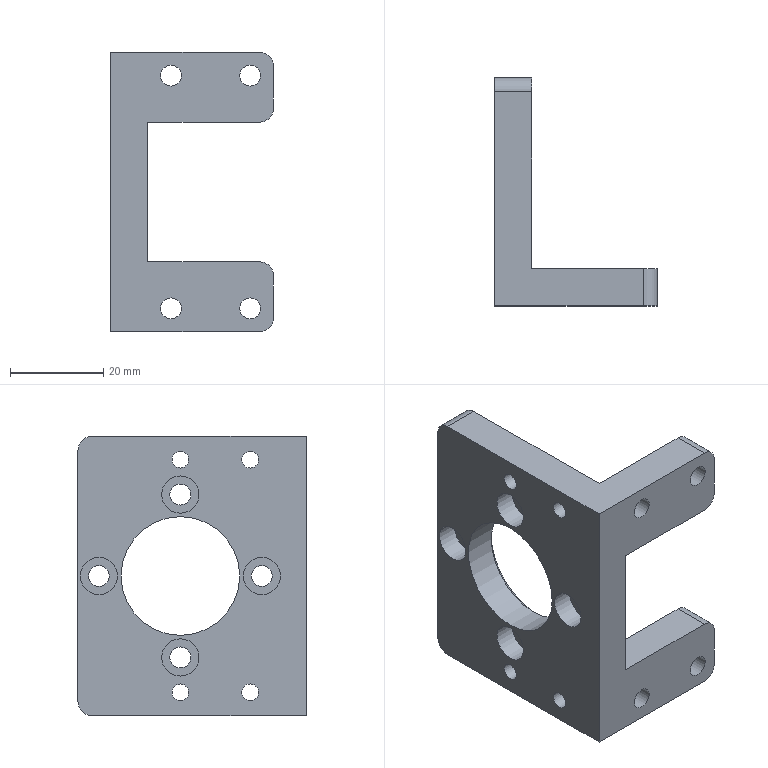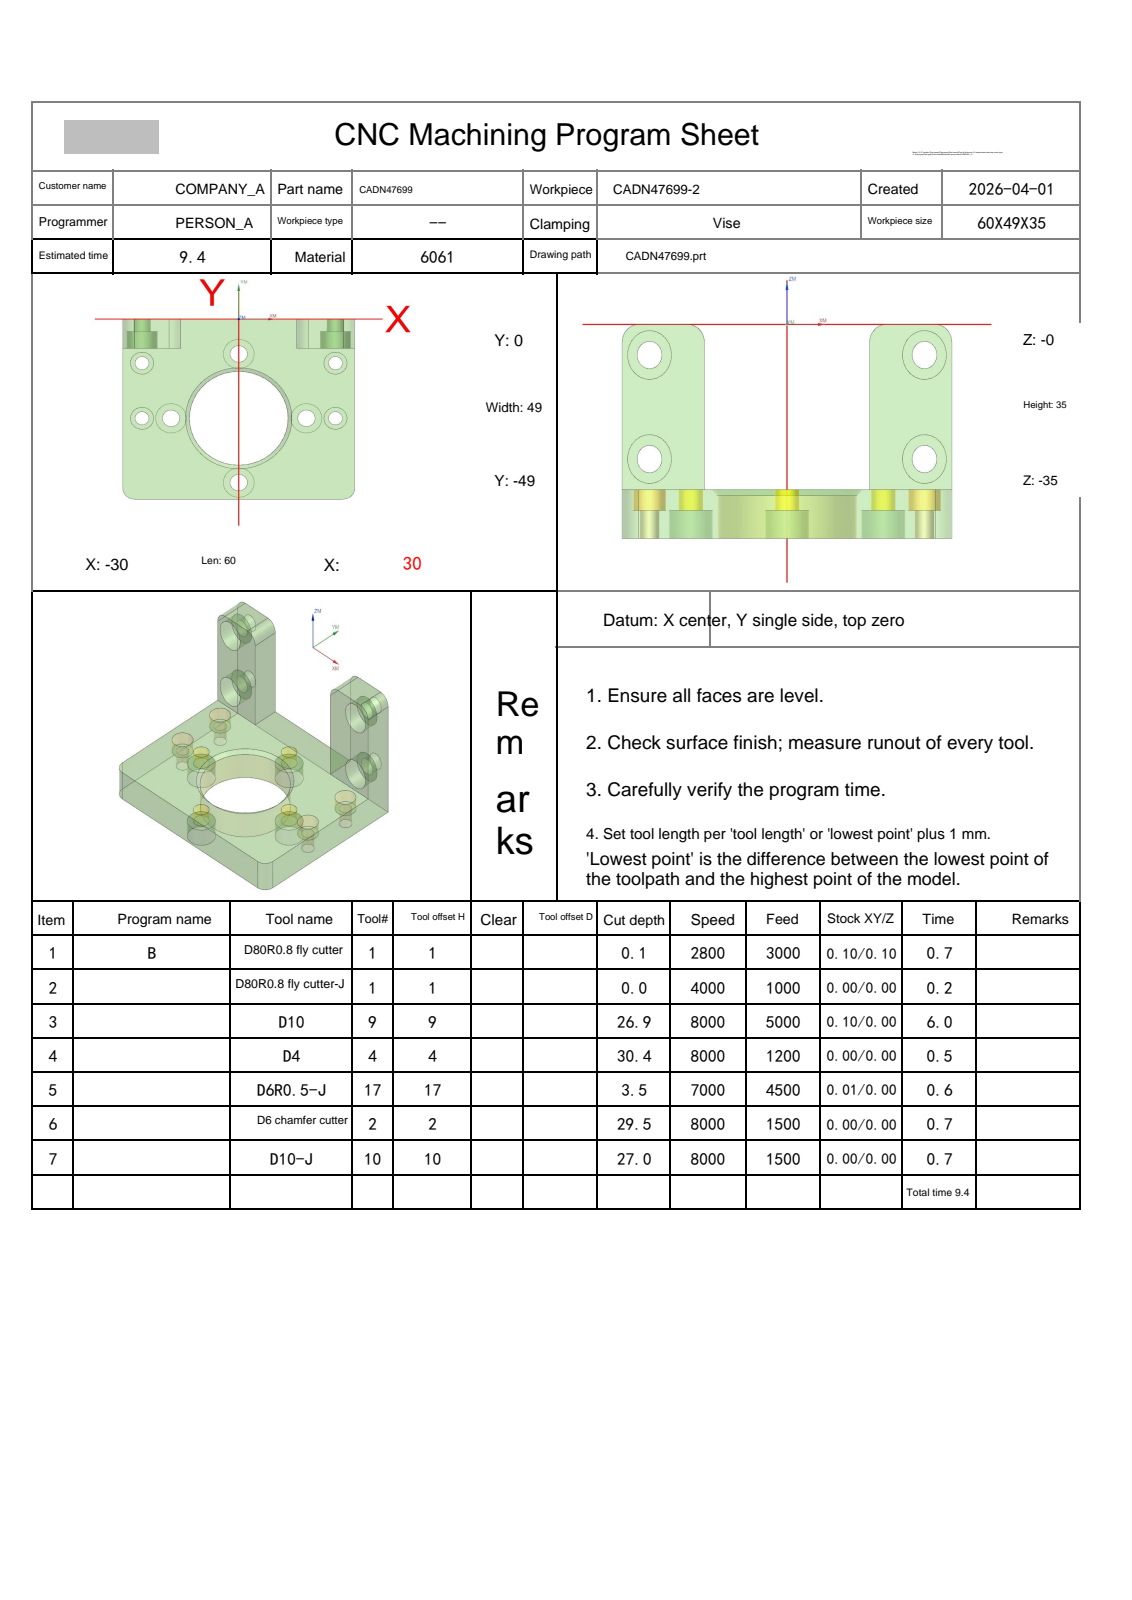NC program | NX | posted by the shop | part box 35 x 49 x 60 mm
Lines 3953 to 5920 of 5920, first 1814 of 1968 lines:
N4 T04 M06
(D4  D=4. R=0. H=04 ce=0.07 di=0.00)
G00 G90 G54 X-25. Y-27. M03 S8000
G43 H04 Z20.
M08
Z-26.7
G03 X-25.465 Y-27.465 I0.0 J-.465 F1200.
X-25. Y-27.93 I.465 J0.0
X-25. Y-27.93 Z-26.9 I0.0 J.93
X-25. Y-27.93 Z-27.1 I0.0 J.93
X-25. Y-27.93 Z-27.3 I0.0 J.93
X-25. Y-27.93 Z-27.5 I0.0 J.93
X-25. Y-27.93 Z-27.7 I0.0 J.93
X-25. Y-27.93 Z-27.9 I0.0 J.93
X-25. Y-27.93 Z-28.1 I0.0 J.93
X-25. Y-27.93 Z-28.3 I0.0 J.93
X-25. Y-27.93 Z-28.5 I0.0 J.93
X-25. Y-27.93 Z-28.7 I0.0 J.93
X-25. Y-27.93 Z-28.9 I0.0 J.93
X-25. Y-27.93 Z-29.1 I0.0 J.93
X-25. Y-27.93 Z-29.3 I0.0 J.93
X-25. Y-27.93 Z-29.5 I0.0 J.93
X-25. Y-27.93 Z-29.7 I0.0 J.93
X-25. Y-27.93 Z-29.9 I0.0 J.93
X-25. Y-27.93 Z-30.1 I0.0 J.93
X-25. Y-27.93 Z-30.3 I0.0 J.93
X-25. Y-26.07 Z-30.4 I0.0 J.93
X-25.93 Y-27. I0.0 J-.93
X-25. Y-27.93 I.93 J0.0
X-24.07 Y-27. I0.0 J.93
X-25. Y-26.07 I-.93 J0.0
X-25.465 Y-26.535 I0.0 J-.465
X-25. Y-27. I.465 J0.0
G00 Z20.
Y-12.
Z-26.7
G03 X-25.465 Y-12.465 I0.0 J-.465
X-25. Y-12.93 I.465 J0.0
X-25. Y-12.93 Z-26.9 I0.0 J.93
X-25. Y-12.93 Z-27.1 I0.0 J.93
X-25. Y-12.93 Z-27.3 I0.0 J.93
X-25. Y-12.93 Z-27.5 I0.0 J.93
X-25. Y-12.93 Z-27.7 I0.0 J.93
X-25. Y-12.93 Z-27.9 I0.0 J.93
X-25. Y-12.93 Z-28.1 I0.0 J.93
X-25. Y-12.93 Z-28.3 I0.0 J.93
X-25. Y-12.93 Z-28.5 I0.0 J.93
X-25. Y-12.93 Z-28.7 I0.0 J.93
X-25. Y-12.93 Z-28.9 I0.0 J.93
X-25. Y-12.93 Z-29.1 I0.0 J.93
X-25. Y-12.93 Z-29.3 I0.0 J.93
X-25. Y-12.93 Z-29.5 I0.0 J.93
X-25. Y-12.93 Z-29.7 I0.0 J.93
X-25. Y-12.93 Z-29.9 I0.0 J.93
X-25. Y-12.93 Z-30.1 I0.0 J.93
X-25. Y-12.93 Z-30.3 I0.0 J.93
X-25. Y-11.07 Z-30.4 I0.0 J.93
X-25.93 Y-12. I0.0 J-.93
X-25. Y-12.93 I.93 J0.0
X-24.07 Y-12. I0.0 J.93
X-25. Y-11.07 I-.93 J0.0
X-25.465 Y-11.535 I0.0 J-.465
X-25. Y-12. I.465 J0.0
G00 Z20.
X25.
Z-26.7
G03 X24.535 Y-12.465 I0.0 J-.465
X25. Y-12.93 I.465 J0.0
X25. Y-12.93 Z-26.9 I0.0 J.93
X25. Y-12.93 Z-27.1 I0.0 J.93
X25. Y-12.93 Z-27.3 I0.0 J.93
X25. Y-12.93 Z-27.5 I0.0 J.93
X25. Y-12.93 Z-27.7 I0.0 J.93
X25. Y-12.93 Z-27.9 I0.0 J.93
X25. Y-12.93 Z-28.1 I0.0 J.93
X25. Y-12.93 Z-28.3 I0.0 J.93
X25. Y-12.93 Z-28.5 I0.0 J.93
X25. Y-12.93 Z-28.7 I0.0 J.93
X25. Y-12.93 Z-28.9 I0.0 J.93
X25. Y-12.93 Z-29.1 I0.0 J.93
X25. Y-12.93 Z-29.3 I0.0 J.93
X25. Y-12.93 Z-29.5 I0.0 J.93
X25. Y-12.93 Z-29.7 I0.0 J.93
X25. Y-12.93 Z-29.9 I0.0 J.93
X25. Y-12.93 Z-30.1 I0.0 J.93
X25. Y-12.93 Z-30.3 I0.0 J.93
X25. Y-11.07 Z-30.4 I0.0 J.93
X24.07 Y-12. I0.0 J-.93
X25. Y-12.93 I.93 J0.0
X25.93 Y-12. I0.0 J.93
X25. Y-11.07 I-.93 J0.0
X24.535 Y-11.535 I0.0 J-.465
X25. Y-12. I.465 J0.0
G00 Z20.
Y-27.
Z-26.7
G03 X24.535 Y-27.465 I0.0 J-.465
X25. Y-27.93 I.465 J0.0
X25. Y-27.93 Z-26.9 I0.0 J.93
X25. Y-27.93 Z-27.1 I0.0 J.93
X25. Y-27.93 Z-27.3 I0.0 J.93
X25. Y-27.93 Z-27.5 I0.0 J.93
X25. Y-27.93 Z-27.7 I0.0 J.93
X25. Y-27.93 Z-27.9 I0.0 J.93
X25. Y-27.93 Z-28.1 I0.0 J.93
X25. Y-27.93 Z-28.3 I0.0 J.93
X25. Y-27.93 Z-28.5 I0.0 J.93
X25. Y-27.93 Z-28.7 I0.0 J.93
X25. Y-27.93 Z-28.9 I0.0 J.93
X25. Y-27.93 Z-29.1 I0.0 J.93
X25. Y-27.93 Z-29.3 I0.0 J.93
X25. Y-27.93 Z-29.5 I0.0 J.93
X25. Y-27.93 Z-29.7 I0.0 J.93
X25. Y-27.93 Z-29.9 I0.0 J.93
X25. Y-27.93 Z-30.1 I0.0 J.93
X25. Y-27.93 Z-30.3 I0.0 J.93
X25. Y-26.07 Z-30.4 I0.0 J.93
X24.07 Y-27. I0.0 J-.93
X25. Y-27.93 I.93 J0.0
X25.93 Y-27. I0.0 J.93
X25. Y-26.07 I-.93 J0.0
X24.535 Y-26.535 I0.0 J-.465
X25. Y-27. I.465 J0.0
G00 Z20.
G00 G90 X-25. Y-27. M03 S8000
Z20.
Z-30.4
G01 X-25.272 Y-27.568 F600.
X-25.302 Y-27.698
G03 X-25. Y-28. I.302 J0.0
X-24. Y-27. I0.0 J1.
X-25. Y-26. I-1. J0.0
X-26. Y-27. I0.0 J-1.
X-25. Y-28. I1. J0.0
X-24.521 Y-27.878 I0.0 J1.
X-24.364 Y-27.613 I-.145 J.265
X-24.489 Y-27.368 I-.302 J0.0
G01 X-25. Y-27.
G00 Z20.
Y-12.
Z-30.4
G01 X-25.272 Y-12.568
X-25.302 Y-12.698
G03 X-25. Y-13. I.302 J0.0
X-24. Y-12. I0.0 J1.
X-25. Y-11. I-1. J0.0
X-26. Y-12. I0.0 J-1.
X-25. Y-13. I1. J0.0
X-24.521 Y-12.878 I0.0 J1.
X-24.364 Y-12.613 I-.145 J.265
X-24.489 Y-12.368 I-.302 J0.0
G01 X-25. Y-12.
G00 Z20.
X25.
Z-30.4
G01 X24.728 Y-12.568
X24.698 Y-12.698
G03 X25. Y-13. I.302 J0.0
X26. Y-12. I0.0 J1.
X25. Y-11. I-1. J0.0
X24. Y-12. I0.0 J-1.
X25. Y-13. I1. J0.0
X25.479 Y-12.878 I0.0 J1.
X25.636 Y-12.613 I-.145 J.265
X25.511 Y-12.368 I-.302 J0.0
G01 X25. Y-12.
G00 Z20.
Y-27.
Z-30.4
G01 X24.728 Y-27.568
X24.698 Y-27.698
G03 X25. Y-28. I.302 J0.0
X26. Y-27. I0.0 J1.
X25. Y-26. I-1. J0.0
X24. Y-27. I0.0 J-1.
X25. Y-28. I1. J0.0
X25.479 Y-27.878 I0.0 J1.
X25.636 Y-27.613 I-.145 J.265
X25.511 Y-27.368 I-.302 J0.0
G01 X25. Y-27.
G00 Z20.
G91 G28 Z0.0
M05
M09
G91 G28 Z0.0
M01
N5 T17 M06
(D6R0.5-J  D=6. R=0.5 H=17 ce=0.01 di=0.00)
G00 G90 G54 X28.911 Y6.347 M03 S7000
G43 H17 Z14.5
M08
Z.493
G01 Z-.007 F4500.
X29.587 Y1.103
X29.729 Y0.0
Y-8.
X29.589 Y-8.912
X29.58 Y-9.105
X29.633 Y-9.103 Z-.011
X29.661 Y-9.102 Z-.015
X29.828 Y-8.
Y0.0
X29.676 Y1.1
X29.721 Z-.019
X29.738 Z-.023
X29.913 Y0.0
Y-8.
X29.723 Y-9.1
X29.773 Z-.028
X29.783 Z-.033
G03 X29.988 Y-8. I-10.112 J2.458
G01 Y0.0
X29.802 Y1.1
X29.866 Z-.038
X29.873 Z-.043
X30.058 Y0.0
Y-8.
G02 X29.847 Y-9.101 I-9.2 J1.191
G01 X29.901 Z-.049
X29.924 Z-.055
G03 X30.131 Y-8. I-7.943 J2.061
G01 Y0.0
X29.957 Y1.1
X30.01 Z-.063
X30.042 Z-.07
X30.205 Y0.0
Y-8.
X30.01 Y-9.101
X30.045 Z-.078
X30.083 Z-.086
X30.282 Y-8.
Y0.0
X30.107 Y1.1
X30.157 Z-.095
X30.179 Z-.104
X30.359 Y0.0
Y-8.
X30.344 Y-8.223
X30.159 Y-9.101
X30.19 Y-9.1 Z-.113
X30.231 Z-.122
X30.413 Y-8.223
X30.426 Y-8.
Y0.0
G03 X30.248 Y1.1 I-20.626 J-2.768
G01 X30.281 Z-.129
X30.3 Z-.135
G02 X30.473 Y0.0 I-19.318 J-3.601
G01 Y-8.
G02 X30.285 Y-9.1 I-6.32 J.513
G01 X30.319 Z-.145
X30.363 Z-.155
X30.528 Y-8.223
X30.539 Y-8.
Y0.0
X30.377 Y1.1
X30.428 Z-.168
X30.476 Y1.101 Z-.181
X30.622 Y0.0
Y-8.
G02 X30.471 Y-9.101 I-30.416 J3.623
G01 X30.526 Y-9.1 Z-.196
X30.574 Z-.211
X30.708 Y-8.
Y0.0
G02 X30.575 Y1.101 I18.741 J2.813
G01 X30.623 Z-.228
X30.661 Y1.1 Z-.244
X30.794 Y0.0
Y-8.
G02 X30.659 Y-9.1 I-88.201 J10.196
G01 X30.709 Z-.261
X30.749 Z-.279
X30.879 Y-8.
Y0.0
X30.75 Y1.1
X30.797 Z-.298
X30.841 Z-.317
G03 X30.965 Y0.0 I15.08 J1.142
G01 Y-8.
G02 X30.839 Y-9.1 I-80.656 J8.64
G01 X30.879 Z-.332
X30.913 Z-.347
G03 X31.03 Y-8. I-78.58 J8.913
G01 Y0.0
G02 X30.915 Y1.1 I16.184 J2.255
G01 X30.967 Z-.368
X31.015 Z-.389
G03 X31.114 Y0.0 I18.175 J1.077
G01 Y-8.
X31.014 Y-9.1
X31.062 Z-.412
X31.104 Z-.434
X31.106 Y-8.912
X31.199 Y-8.
Y0.0
G02 X31.105 Y1.1 I9.034 J1.321
G01 X31.15 Z-.458
X31.185 Z-.482
G03 X31.283 Y0.0 I8.509 J.204
G01 Y-8.
X31.186 Y-8.912
X31.184 Y-9.1
X31.231 Z-.507
X31.267 Z-.532
X31.365 Y-8.
Y0.0
G02 X31.268 Y1.1 I9.408 J1.387
G01 X31.315 Z-.559
X31.355 Z-.585
X31.358 Y.737
G02 X31.447 Y0.0 I-3.779 J-.832
G01 Y-8.
X31.354 Y-9.1
X31.4 Z-.611
X31.439 Z-.637
G02 X31.524 Y-8. I15.841 J-.662
G01 Y0.0
G02 X31.44 Y1.1 I8.494 J1.204
G01 X31.489 Z-.666
X31.525 Y1.101 Z-.694
Y1.094
G03 X31.602 Y0.0 I7.765 J0.0
G01 Y-8.
X31.525 Y-9.1
X31.569 Z-.724
X31.606 Z-.754
G02 X31.68 Y-8. I15.314 J-.479
G01 Y0.0
G02 X31.607 Y1.085 I8.046 J1.085
G01 Y1.101
X31.645 Y1.1 Z-.785
X31.68 Z-.816
G03 X31.757 Y0.0 I10.352 J.166
G01 Y-8.
G03 X31.679 Y-9.1 I17.687 J-1.803
G01 X31.719 Z-.848
X31.756 Z-.88
Y-8.912
X31.831 Y-8.
Y0.0
G02 X31.756 Y1.1 I10.366 J1.261
G01 X31.795 Z-.914
X31.833 Z-.947
G03 X31.904 Y0.0 I10.581 J.129
G01 Y-8.
X31.834 Y-8.912
X31.832 Y-9.1
X31.874 Z-.981
X31.912 Z-1.015
X31.914 Y-8.912
X31.975 Y-8.
Y0.0
G02 X31.913 Y1.101 I10.911 J1.164
G01 X31.949 Z-1.051
X31.98 Z-1.086
G03 X32.044 Y0.0 I10.181 J.042
G01 Y-8.
G03 X31.979 Y-9.1 I12.2 J-1.277
G01 X32.018 Z-1.122
X32.044 Z-1.159
X32.058 Y-8.567
G03 X32.112 Y-8. I-3.108 J.58
G01 Y0.0
X32.111 Y.048
X32.046 Y.737
X32.045 Y1.1
X32.08 Z-1.196
X32.111 Z-1.233
G03 X32.177 Y0.0 I10.427 J.069
G01 Y-8.
G03 X32.11 Y-9.1 I14.904 J-1.459
G01 X32.145 Z-1.272
X32.175 Z-1.31
G02 X32.24 Y-8. I15.396 J-.354
G01 Y0.0
G02 X32.177 Y1.1 I10.242 J1.142
G01 X32.211 Y1.101 Z-1.349
X32.244 Z-1.388
G03 X32.301 Y0.0 I11.649 J.057
G01 Y-8.
G03 X32.242 Y-9.1 I19.264 J-1.583
G01 X32.277 Z-1.428
X32.302 Z-1.468
G02 X32.36 Y-8. I12.798 J-.123
G01 Y0.0
G02 X32.301 Y.94 I7.512 J.94
G01 X32.303 Y1.101
X32.335 Y1.1 Z-1.509
X32.356 Z-1.55
G03 X32.417 Y0.0 I10.101 J.002
G01 Y-8.
G02 X32.366 Y-8.567 I-4.632 J.124
G01 X32.355 Y-9.1
X32.388 Z-1.592
X32.409 Z-1.634
X32.421 Y-8.567
G03 X32.471 Y-8. I-4.52 J.683
G01 Y0.0
X32.411 Y.737
Y1.1
X32.44 Z-1.676
X32.464 Z-1.719
G03 X32.523 Y0.0 I10.304 J.003
G01 Y-8.
G02 X32.473 Y-8.567 I-6.092 J.246
G01 X32.462 Y-9.1
X32.492 Z-1.762
X32.511 Z-1.805
X32.523 Y-8.567
G03 X32.572 Y-8. I-6.129 J.814
G01 Y0.0
G02 X32.513 Y1.1 I10.22 J1.101
G01 X32.546 Z-1.849
X32.563 Y1.101 Z-1.893
X32.56 Y.96
G03 X32.569 Y.727 I3.192 J0.0
G01 X32.619 Y.048
Y0.0
Y-8.
G02 X32.574 Y-8.567 I-4.739 J.091
G01 X32.561 Y-9.1
X32.591 Z-1.938
X32.612 Z-1.982
G02 X32.664 Y-8. I14.571 J-.134
G01 Y0.0
G02 X32.614 Y1.08 I11.661 J1.08
G01 Y1.101
X32.635 Z-2.028
X32.653 Z-2.073
Y1.017
G03 X32.706 Y0.0 I9.751 J0.0
G01 Y-8.
G03 X32.652 Y-9.1 I11.168 J-1.101
G01 X32.673 Z-2.119
X32.69 Z-2.165
G02 X32.745 Y-8. I11.063 J-.008
G01 Y0.0
G02 X32.69 Y1.012 I9.315 J1.012
G01 X32.691 Y1.101
X32.711 Y1.1 Z-2.211
X32.729 Z-2.257
Y1.034
G03 X32.782 Y0.0 I10.105 J0.0
G01 Y-8.
G02 X32.738 Y-8.567 I-7.023 J.256
G01 X32.728 Y-9.1
X32.75 Z-2.304
X32.767 Z-2.351
G02 X32.816 Y-8. I17.958 J-.257
G01 Y0.0
G02 X32.768 Y1.096 I12.454 J1.096
G01 Y1.1
X32.788 Z-2.399
X32.802 Z-2.446
X32.801 Y.965
G03 X32.848 Y0.0 I10.073 J0.0
G01 Y-8.
G03 X32.801 Y-9.044 I11.783 J-1.044
G01 X32.802 Y-9.097
X32.828 Y-9.089 Z-2.542
Y-9.076
G02 X32.876 Y-8. I11.939 J0.0
G01 Y0.0
G02 X32.825 Y1.025 I10.281 J1.025
G01 X32.826 Y1.1
X32.841 Z-2.59
X32.849 Z-2.638
G03 X32.902 Y0.0 I12.284 J.044
G01 Y-8.
G02 X32.86 Y-8.567 I-5.644 J.138
G01 X32.854 Y-9.081
X32.881 Y-9.072 Z-2.736
X32.886 Y-8.567
G03 X32.925 Y-8. I-7.188 J.788
G01 Y0.0
G02 X32.873 Y1.1 I16.669 J1.353
G01 X32.888 Z-2.784
X32.896 Z-2.833
G03 X32.946 Y0.0 I21.579 J.424
G01 Y-8.
G03 X32.906 Y-9.015 I12.925 J-1.015
G01 Y-9.064
X32.928 Y-9.056 Z-2.932
X32.931 Y-8.567
X32.964 Y-8.
Y0.0
G02 X32.92 Y1.1 I19.869 J1.343
G01 X32.934 Z-2.981
X32.944 Z-3.031
X32.943 Y1.089
X32.978 Y0.0
Y-8.
G03 X32.95 Y-8.928 I14.896 J-.928
G01 Y-9.048
X32.968 Y-9.039 Z-3.13
X32.967 Y-8.871
G02 X32.99 Y-8. I16.225 J0.0
G01 Y0.0
X32.987 Y.048
X32.962 Y1.096
X32.976 Z-3.222
X32.974 Y1.091
X32.993 Y.048
X32.999 Y0.0
Y-8.
G03 X32.982 Y-8.843 I20.646 J-.843
G01 X32.983 Y-9.031
X32.992 Y-9.023 Z-3.315
X32.991 Y-8.83
G02 X33.005 Y-8. I24.869 J0.0
G01 Y0.0
X32.988 Y1.091
X32.989 Y1.097
X32.994 Z-3.361
X33.001 Y1.098 Z-3.407
X33.006 Y.048
X33.009 Y0.0
Y-8.
X33.001 Y-9.015
X33.008 Y-9.007 Z-3.5
X33.009 Y-8.912
X33.01 Y-8.
Y0.0
Y1.098
G00 Z14.5
X15.444 Y-14.037
Z.493
G01 Z-.007
X15.43 Y-9.1
Y-8.912
X15.271 Y-8.
Y0.0
G02 X15.438 Y1.1 I42.775 J-5.935
G01 X15.371 Z-.015
G03 X15.172 Y0.0 I21.874 J-4.539
G01 Y-8.
X15.353 Y-8.912
X15.354 Y-9.1
X15.279 Z-.019
X15.268 Z-.023
X15.087 Y-8.
Y0.0
G02 X15.295 Y1.1 I4.405 J-.262
G01 X15.212 Z-.033
G03 X15.012 Y0.0 I10.091 J-2.401
G01 Y-8.
X15.174 Y-9.1
X15.132 Z-.038
X15.112 Z-.043
X14.942 Y-8.
Y0.0
G02 X15.136 Y1.1 I15.778 J-2.212
G01 X15.097 Z-.049
X15.079 Z-.055
G03 X14.869 Y0.0 I6.496 J-1.81
G01 Y-8.
X15.051 Y-9.1
X14.99 Z-.063
X14.981 Z-.07
X14.795 Y-8.
Y0.0
G02 X15.014 Y1.1 I4.199 J-.263
G01 X14.938 Z-.086
G03 X14.718 Y0.0 I3.488 J-1.268
G01 Y-8.
X14.9 Y-9.1
X14.844 Z-.095
X14.81 Z-.104
X14.641 Y-8.
Y0.0
G02 X14.853 Y1.1 I4.859 J-.367
G01 X14.777 Z-.122
G03 X14.574 Y0.0 I5.8 J-1.634
G01 Y-8.
X14.74 Y-8.912
X14.745 Y-9.1
X14.696 Z-.135
X14.527 Y-8.
Y0.0
G02 X14.722 Y1.1 I6.572 J-.598
G01 X14.681 Z-.145
X14.642 Z-.155
G03 X14.461 Y0.0 I17.784 J-3.481
G01 Y-8.
X14.624 Y-9.1
X14.572 Z-.168
X14.525 Z-.181
G02 X14.378 Y-8. I19.215 J3.122
G01 Y0.0
G02 X14.531 Y1.1 I17.771 J-1.916
G01 X14.473 Z-.196
X14.428 Z-.211
X14.292 Y0.0
Y-8.
X14.427 Y-8.912
X14.429 Y-9.1
X14.377 Z-.228
X14.346 Z-.244
G03 X14.206 Y-8. I-122.834 J-15.056
G01 Y0.0
X14.345 Y1.1
X14.291 Z-.261
X14.257 Z-.279
X14.121 Y0.0
Y-8.
G02 X14.258 Y-9.1 I-165.869 J-21.194
G01 X14.203 Z-.298
X14.162 Z-.317
G03 X14.035 Y-8. I-84.189 J-9.168
G01 Y0.0
G03 X14.161 Y1.1 I-45.92 J5.804
G01 X14.121 Z-.332
X14.085 Z-.347
X13.97 Y0.0
Y-8.
X14.084 Y-8.912
X14.086 Y-9.1
X14.033 Z-.368
X13.986 Z-.389
X13.983 Y-8.912
X13.886 Y-8.
Y0.0
X13.984 Y1.101
X13.938 Z-.412
X13.895 Z-.434
G02 X13.801 Y0.0 I-10.174 J.309
G01 Y-8.
X13.896 Y-9.1
X13.849 Z-.458
X13.815 Z-.482
X13.717 Y-8.
Y0.0
G02 X13.81 Y.737 I4.024 J-.133
G01 X13.813 Y1.1
X13.769 Z-.507
X13.731 Z-.532
G02 X13.635 Y0.0 I-8.376 J.178
G01 Y-8.
X13.73 Y-8.912
X13.732 Y-9.1
X13.685 Z-.559
X13.65 Z-.585
X13.647 Y-8.912
X13.553 Y-8.
Y0.0
G03 X13.648 Y1.1 I-7.852 J1.233
G01 X13.6 Z-.611
X13.566 Z-.637
G02 X13.476 Y0.0 I-8.742 J.157
G01 Y-8.
X13.564 Y-8.912
X13.567 Y-9.1
X13.511 Z-.666
X13.478 Z-.694
X13.475 Y-8.912
X13.398 Y-8.
Y0.0
G03 X13.476 Y1.1 I-11.764 J1.393
G01 X13.431 Z-.724
X13.392 Z-.754
G02 X13.32 Y0.0 I-10.331 J.131
G01 Y-8.
G02 X13.394 Y-9.1 I-11.712 J-1.341
G01 X13.355 Z-.785
X13.321 Z-.816
G03 X13.243 Y-8. I-16.596 J-.62
G01 Y0.0
G03 X13.32 Y1.1 I-10.704 J1.296
G01 X13.281 Z-.848
X13.245 Z-.88
G02 X13.169 Y0.0 I-10.595 J.177
G01 Y-8.
G02 X13.246 Y-9.1 I-13.853 J-1.524
G01 X13.205 Z-.914
X13.168 Z-.947
G03 X13.096 Y-8. I-14.365 J-.391
G01 Y0.0
G03 X13.167 Y1.1 I-10.583 J1.234
G01 X13.126 Z-.981
X13.087 Z-1.015
G02 X13.025 Y0.0 I-11.249 J.079
G01 Y-8.
G02 X13.088 Y-9.1 I-13.727 J-1.338
G01 X13.051 Z-1.051
X13.023 Z-1.086
G03 X12.956 Y-8. I-13.064 J-.25
G01 Y0.0
G03 X13.022 Y1.1 I-10.138 J1.164
G01 X12.983 Z-1.122
X12.958 Z-1.159
Y.737
X12.888 Y0.0
Y-8.
G03 X12.946 Y-8.567 I2.901 J.007
G01 X12.959 Y-9.1
X12.92 Z-1.196
X12.894 Z-1.233
X12.88 Y-8.567
G02 X12.823 Y-8. I3.617 J.651
G01 Y0.0
X12.892 Y.737
X12.893 Y1.1
X12.855 Z-1.272
X12.826 Z-1.31
G02 X12.76 Y0.0 I-10.397 J.071
G01 Y-8.
G03 X12.813 Y-8.567 I3.905 J.08
G01 X12.827 Y-9.1
X12.789 Z-1.349
X12.758 Z-1.388
G03 X12.699 Y-8. I-18.513 J-.451
G01 Y0.0
G03 X12.757 Y1.1 I-11.537 J1.162
G01 X12.723 Z-1.428
X12.698 Z-1.468
Y1.071
G02 X12.64 Y0.0 I-9.936 J0.0
G01 Y-8.
G02 X12.699 Y-9.1 I-12.945 J-1.245
G01 X12.666 Z-1.509
X12.645 Z-1.55
X12.634 Y-8.567
G02 X12.583 Y-8. I4.371 J.675
G01 Y0.0
G03 X12.644 Y1.1 I-10.138 J1.112
G01 X12.612 Z-1.592
X12.589 Z-1.634
Y.737
X12.529 Y0.0
Y-8.
G03 X12.579 Y-8.567 I4.241 J.086
G01 X12.591 Y-9.1
X12.56 Z-1.676
X12.538 Z-1.719
X12.527 Y-8.567
G02 X12.477 Y-8. I6.185 J.824
G01 Y0.0
G03 X12.537 Y1.1 I-10.255 J1.104
G01 X12.508 Z-1.762
X12.486 Z-1.805
G02 X12.428 Y0.0 I-10.51 J.008
G01 Y-8.
G03 X12.476 Y-8.567 I6.25 J.244
G01 X12.488 Y-9.1
X12.454 Z-1.849
X12.437 Z-1.893
X12.424 Y-8.567
X12.385 Y-8.106
X12.381 Y-8.
Y0.0
X12.382 Y.048
X12.429 Y.734
G03 X12.438 Y.975 I-3.457 J.24
G01 X12.435 Y1.1
X12.409 Z-1.938
X12.384 Z-1.982
X12.386 Y.925
G02 X12.336 Y0.0 I-8.688 J0.0
G01 Y-8.
G02 X12.384 Y-9.09 I-12.278 J-1.09
G01 Y-9.1
X12.365 Z-2.028
X12.348 Z-2.073
Y-9.098
G03 X12.294 Y-8. I-11.186 J0.0
G01 Y0.0
G03 X12.347 Y1.01 I-9.57 J1.01
G01 Y1.1
X12.327 Y1.101 Z-2.119
X12.309 Z-2.165
X12.31 Y1.007
G02 X12.255 Y0.0 I-9.294 J0.0
G01 Y-8.
G02 X12.31 Y-9.1 I-11.451 J-1.129
G01 X12.289 Z-2.211
X12.272 Z-2.257
X12.262 Y-8.567
G02 X12.218 Y-8. I6.105 J.756
G01 Y0.0
G03 X12.271 Y1.032 I-10.045 J1.032
G01 Y1.101
X12.25 Y1.102 Z-2.304
X12.232 Z-2.351
Y1.064
G02 X12.184 Y0.0 I-11.823 J0.0
G01 Y-8.
X12.223 Y-8.567
X12.233 Y-9.1
X12.216 Z-2.399
X12.201 Z-2.446
G03 X12.152 Y-8. I-15. J-.105
G01 Y0.0
G03 X12.199 Y.983 I-10.269 J.983
G01 Y1.101
X12.184 Z-2.494
X12.172 Z-2.542
Y1.007
G02 X12.124 Y0.0 I-10.458 J0.0
G01 Y-8.
G03 X12.164 Y-8.567 I5.743 J.127
G01 X12.176 Y-9.1
X12.159 Z-2.59
X12.151 Z-2.638
G03 X12.098 Y-8. I-16.684 J-.261
G01 Y0.0
G03 X12.145 Y1.032 I-11.243 J1.032
G01 Y1.101
X12.13 Z-2.687
X12.119 Z-2.736
X12.12 Y.957
G02 X12.075 Y0.0 I-10.087 J0.0
G01 Y-8.
G02 X12.126 Y-9.1 I-15.582 J-1.287
G01 X12.112 Z-2.784
X12.104 Z-2.833
G03 X12.054 Y-8. I-17.218 J-.233
G01 Y0.0
G03 X12.098 Y.937 I-10.07 J.937
G01 X12.096 Y1.101
X12.077 Y1.1 Z-2.883
X12.073 Z-2.932
X12.074 Y.943
G02 X12.036 Y0.0 I-11.72 J0.0
G01 Y-8.
G02 X12.082 Y-9.1 I-23.271 J-1.516
G01 X12.066 Z-2.981
X12.06 Z-3.031
X12.022 Y-8.
Y0.0
G03 X12.051 Y.966 I-15.624 J.966
G01 Y1.1
X12.039 Z-3.08
X12.033 Y1.099 Z-3.13
X12.034 Y.965
G02 X12.01 Y0.0 I-19.39 J0.0
G01 Y-8.
G02 X12.038 Y-9.099 I-27.238 J-1.25
G01 X12.026 Y-9.087 Z-3.222
G03 X12.001 Y-8. I-143.334 J-2.736
G01 Y0.0
G03 X12.022 Y1.053 I-26.254 J1.053
G01 Y1.099
X12.011 Y1.098 Z-3.269
Z-3.315
X12. Y.048
X11.995 Y0.0
Y-8.
X12.014 Y-9.075
X12.001 Y-9.064 Z-3.407
X11.991 Y-8.
Y0.0
X11.995 Y.048
X12. Y1.097
X11.991 Z-3.5
X11.99 Y0.0
Y-8.
Y-8.912
X11.992 Y-9.052
G00 Z14.5
X-14.998 Y5.777
Z.493
G01 Z-.007
X-15.429 Y1.1
X-15.271 Y0.0
Y-8.
X-15.435 Y-9.1
X-15.366 Y-9.101 Z-.015
X-15.352 Y-8.912
X-15.172 Y-8.
Y0.0
X-15.353 Y1.1
X-15.279 Z-.019
X-15.265 Z-.023
G02 X-15.087 Y0.0 I-16.61 J-3.253
G01 Y-8.
X-15.286 Y-9.101
X-15.229 Y-9.102 Z-.028
X-15.2 Z-.033
X-15.012 Y-8.
Y0.0
X-15.17 Y1.1
X-15.132 Z-.038
X-15.11 Z-.043
X-15.109 Y1.082
X-14.942 Y0.0
Y-8.
X-15.129 Y-9.101
X-15.099 Z-.049
X-15.069 Z-.055
X-14.869 Y-8.
Y0.0
X-15.05 Y1.1
X-14.99 Z-.063
X-14.981 Z-.07
X-14.795 Y0.0
Y-8.
X-15.001 Y-9.102
X-14.954 Z-.078
X-14.922 Z-.086
G03 X-14.718 Y-8. I-8.055 J2.06
G01 Y0.0
G03 X-14.901 Y1.1 I-16.261 J-2.13
G01 X-14.844 Z-.095
X-14.811 Z-.104
X-14.641 Y0.0
Y-8.
X-14.835 Y-9.103
X-14.81 Y-9.102 Z-.113
X-14.763 Y-9.101 Z-.122
X-14.574 Y-8.
Y0.0
X-14.745 Y1.1
X-14.696 Z-.135
X-14.527 Y0.0
Y-8.
G02 X-14.71 Y-9.101 I-11.255 J1.312
G01 X-14.681 Z-.145
X-14.634 Y-9.1 Z-.155
X-14.461 Y-8.
Y0.0
X-14.623 Y1.1
X-14.572 Z-.168
X-14.524 Z-.181
X-14.378 Y0.0
Y-8.
G02 X-14.529 Y-9.1 I-30.237 J3.597
G01 X-14.473 Z-.196
X-14.429 Z-.211
X-14.292 Y-8.
Y0.0
X-14.427 Y1.1
X-14.377 Z-.228
X-14.345 Z-.244
X-14.344 Y1.082
X-14.206 Y0.0
Y-8.
G03 X-14.347 Y-9.1 I71.306 J-9.64
G01 X-14.291 Z-.261
X-14.258 Z-.279
G02 X-14.121 Y-8. I29.237 J-3.083
G01 Y0.0
G02 X-14.256 Y1.1 I42.197 J5.758
G01 X-14.203 Z-.298
X-14.161 Z-.317
G03 X-14.035 Y0.0 I32.29 J3.131
G01 Y-8.
X-14.114 Y-8.651
X-14.157 Y-8.797
X-14.162 Y-9.1
X-14.121 Z-.332
X-14.086 Z-.347
G03 X-13.97 Y-8. I-82.796 J9.312
G01 Y0.0
X-14.085 Y1.1
X-14.033 Y1.101 Z-.368
X-13.984 Z-.389
X-13.886 Y0.0
Y-8.
X-13.986 Y-9.1
X-13.938 Z-.412
X-13.896 Z-.434
X-13.801 Y-8.
Y0.0
G02 X-13.895 Y1.101 I10.081 J1.41
G01 X-13.85 Y1.1 Z-.458
X-13.813 Z-.482
X-13.81 Y.737
G02 X-13.717 Y0.0 I-3.931 J-.871
G01 Y-8.
X-13.815 Y-9.1
X-13.769 Z-.507
X-13.732 Z-.532
X-13.73 Y-8.912
X-13.635 Y-8.
Y0.0
G02 X-13.731 Y1.1 I8.28 J1.278
G01 X-13.685 Z-.559
X-13.648 Z-.585
G03 X-13.553 Y0.0 I7.947 J.133
G01 Y-8.
X-13.647 Y-8.912
X-13.65 Y-9.1
X-13.6 Z-.611
X-13.567 Z-.637
X-13.564 Y-8.912
X-13.476 Y-8.
Y0.0
G02 X-13.566 Y1.1 I8.652 J1.257
G01 X-13.512 Z-.666
X-13.476 Z-.694
G03 X-13.398 Y0.0 I11.842 J.293
G01 Y-8.
X-13.478 Y-9.1
X-13.431 Z-.724
X-13.394 Z-.754
X-13.391 Y-8.912
X-13.32 Y-8.
Y0.0
G02 X-13.392 Y1.1 I10.258 J1.231
G01 X-13.355 Z-.785
X-13.32 Z-.816
G03 X-13.243 Y0.0 I10.78 J.196
G01 Y-8.
G03 X-13.321 Y-9.1 I16.518 J-1.72
G01 X-13.281 Z-.848
X-13.246 Z-.88
G02 X-13.169 Y-8. I13.93 J-.424
G01 Y0.0
G02 X-13.245 Y1.1 I10.52 J1.277
G01 X-13.205 Z-.914
X-13.167 Z-.947
G03 X-13.096 Y0.0 I10.654 J.134
G01 Y-8.
X-13.166 Y-8.912
X-13.168 Y-9.1
X-13.126 Z-.981
X-13.088 Z-1.015
G02 X-13.025 Y-8. I13.79 J-.238
G01 Y0.0
G02 X-13.087 Y1.1 I11.188 J1.179
G01 X-13.051 Z-1.051
X-13.022 Z-1.086
G03 X-12.956 Y0.0 I10.205 J.064
G01 Y-8.
G03 X-13.023 Y-9.1 I12.996 J-1.349
G01 X-12.983 Z-1.122
X-12.959 Z-1.159
X-12.946 Y-8.567
G03 X-12.888 Y-8. I-2.844 J.574
G01 Y0.0
X-12.958 Y.737
Y1.1
X-12.92 Z-1.196
X-12.893 Z-1.233
X-12.892 Y.737
X-12.823 Y0.0
Y-8.
G02 X-12.88 Y-8.567 I-3.674 J.084
G01 X-12.894 Y-9.1
X-12.855 Z-1.272
X-12.827 Z-1.31
X-12.813 Y-8.567
G03 X-12.76 Y-8. I-3.851 J.647
G01 Y0.0
G02 X-12.826 Y1.1 I10.331 J1.171
G01 X-12.789 Z-1.349
X-12.757 Z-1.388
G03 X-12.699 Y0.0 I11.595 J.062
G01 Y-8.
G03 X-12.758 Y-9.1 I18.453 J-1.551
G01 X-12.723 Z-1.428
X-12.699 Z-1.468
G02 X-12.64 Y-8. I13.004 J-.145
G01 Y0.0
G02 X-12.698 Y1.071 I9.878 J1.071
G01 Y1.1
X-12.663 Z-1.509
X-12.644 Z-1.55
G03 X-12.583 Y0.0 I10.199 J.012
G01 Y-8.
G02 X-12.634 Y-8.567 I-4.421 J.108
G01 X-12.645 Y-9.1
X-12.612 Z-1.592
X-12.591 Z-1.634
X-12.579 Y-8.567
G03 X-12.529 Y-8. I-4.191 J.653
G01 Y0.0
X-12.589 Y.737
Y1.1
X-12.56 Z-1.676
X-12.537 Z-1.719
G03 X-12.477 Y0.0 I10.315 J.004
G01 Y-8.
G02 X-12.527 Y-8.567 I-6.234 J.257
G01 X-12.538 Y-9.1
X-12.508 Z-1.762
X-12.488 Z-1.805
X-12.476 Y-8.567
G03 X-12.428 Y-8. I-6.202 J.812
G01 Y0.0
G02 X-12.486 Y1.1 I10.451 J1.108
G01 X-12.454 Z-1.849
X-12.435 Z-1.893
X-12.438 Y.975
G03 X-12.429 Y.734 I3.466 J0.0
G01 X-12.382 Y.048
X-12.381 Y0.0
Y-8.
X-12.385 Y-8.106
X-12.424 Y-8.567
X-12.437 Y-9.1
X-12.409 Z-1.938
X-12.384 Z-1.982
Y-9.09
G02 X-12.336 Y-8. I12.326 J0.0
G01 Y0.0
G02 X-12.386 Y.925 I8.639 J.925
G01 X-12.384 Y1.1
X-12.365 Z-2.028
X-12.347 Z-2.073
Y1.01
G03 X-12.294 Y0.0 I9.624 J0.0
G01 Y-8.
G03 X-12.348 Y-9.098 I11.132 J-1.098
G01 Y-9.1
X-12.327 Z-2.119
X-12.31 Z-2.165
G02 X-12.255 Y-8. I11.506 J-.029
G01 Y0.0
G02 X-12.31 Y1.007 I9.242 J1.007
G01 X-12.309 Y1.101
X-12.289 Z-2.211
X-12.271 Y1.102 Z-2.257
Y1.032
G03 X-12.218 Y0.0 I10.104 J0.0
G01 Y-8.
G02 X-12.262 Y-8.567 I-6.148 J.189
G01 X-12.272 Y-9.1
X-12.25 Z-2.304
X-12.233 Z-2.351
X-12.223 Y-8.567
X-12.184 Y-8.
Y0.0
G02 X-12.232 Y1.065 I11.791 J1.065
G01 Y1.102
X-12.216 Z-2.399
X-12.2 Z-2.446
Y1.007
G03 X-12.152 Y0.0 I10.635 J0.0
G01 Y-8.
X-12.193 Y-8.567
X-12.2 Y-9.1
X-12.184 Z-2.494
X-12.173 Z-2.542
X-12.167 Y-8.567
G03 X-12.124 Y-8. I-4.993 J.665
G01 Y0.0
G02 X-12.175 Y1.084 I11.407 J1.084
G01 Y1.102
X-12.159 Z-2.59
X-12.15 Z-2.638
G03 X-12.098 Y0.0 I13.348 J.083
G01 Y-8.
X-12.14 Y-8.567
X-12.146 Y-9.1
X-12.13 Z-2.687
X-12.12 Z-2.736
Y-9.021
G02 X-12.075 Y-8. I11.376 J0.0
G01 Y0.0
G02 X-12.125 Y1.102 I12.882 J1.145
G01 X-12.112 Y1.101 Z-2.784
X-12.103 Z-2.833
G03 X-12.054 Y0.0 I14.849 J.112
G01 Y-8.
G03 X-12.098 Y-9.093 I13.618 J-1.093
G01 Y-9.1
X-12.077 Z-2.883
X-12.075 Z-2.932
G02 X-12.036 Y-8. I17.949 J-.086
G01 Y0.0
G02 X-12.081 Y1.101 I22.156 J1.456
G01 X-12.069 Z-2.981
X-12.059 Y1.1 Z-3.031
G03 X-12.022 Y0.0 I48.003 J1.096
G01 Y-8.
G03 X-12.053 Y-9.055 I17.705 J-1.055
G01 Y-9.1
X-12.034 Y-9.094 Z-3.13
G02 X-12.036 Y-8.878 I14.652 J.216
X-12.01 Y-8. I14.654 J0.0
G01 Y0.0
G02 X-12.038 Y1.1 I22.16 J1.112
G01 X-12.029 Y1.099 Z-3.176
X-12.025 Z-3.222
X-12.006 Y.048
X-12.001 Y0.0
Y-8.
G03 X-12.025 Y-8.862 I15.67 J-.862
X-12.023 Y-9.082 I15.694 J0.0
G01 X-12.012 Y-9.071 Z-3.315
G02 X-12.013 Y-8.862 I20.556 J.209
X-11.995 Y-8. I20.557 J0.0
G01 Y0.0
X-12. Y.048
X-12.013 Y1.099
X-12.007 Y1.098 Z-3.361
X-12.001 Z-3.407
X-11.995 Y.048
X-11.991 Y0.0
Y-8.
X-12.001 Y-9.06
X-11.992 Y-9.048 Z-3.5
X-11.99 Y-8.912
Y-8.
Y0.0
X-11.991 Y1.097
G00 Z14.5
X-29.549 Y-14.04
Z.493
G01 Z-.007
X-29.586 Y-9.101
X-29.588 Y-8.912
X-29.729 Y-8.
Y0.0
X-29.581 Y1.106
X-29.633 Y1.103 Z-.011
X-29.663 Y1.102 Z-.015
G02 X-29.828 Y0.0 I-9.561 J.871
G01 Y-8.
X-29.678 Y-8.912
X-29.675 Y-9.1
X-29.721 Z-.019
X-29.736 Z-.023
X-29.738 Y-8.912
X-29.913 Y-8.
Y0.0
G02 X-29.724 Y1.1 I55.074 J-8.924
G01 X-29.773 Z-.028
X-29.781 Z-.033
G03 X-29.988 Y0.0 I11.93 J-2.814
G01 Y-8.
X-29.803 Y-8.912
X-29.801 Y-9.1
X-29.866 Z-.038
X-29.871 Z-.043
G03 X-30.058 Y-8. I-42.081 J-6.593
G01 Y0.0
G02 X-29.844 Y1.1 I11.09 J-1.589
G01 X-29.902 Z-.049
X-29.918 Z-.055
G03 X-30.131 Y0.0 I9.84 J-2.471
G01 Y-8.
X-29.954 Y-9.1
X-30.01 Z-.063
X-30.04 Z-.07
X-30.205 Y-8.
Y0.0
G02 X-30.004 Y1.1 I9.073 J-1.087
G01 X-30.048 Z-.078
X-30.078 Z-.086
G03 X-30.282 Y0.0 I3.94 J-1.299
G01 Y-8.
X-30.105 Y-9.1
X-30.157 Z-.095
X-30.178 Z-.104
X-30.18 Y-8.912
X-30.359 Y-8.
Y0.0
G02 X-30.152 Y1.1 I5.212 J-.411
G01 X-30.223 Z-.122
G03 X-30.426 Y0.0 I4.197 J-1.342
G01 Y-8.
X-30.362 Y-8.567
G02 X-30.244 Y-9.027 I-.834 J-.46
G01 X-30.247 Y-9.1
X-30.281 Z-.129
X-30.299 Z-.135
G02 X-30.473 Y-8. I11.802 J2.433
G01 Y0.0
G02 X-30.278 Y1.1 I5.317 J-.378
G01 X-30.358 Z-.155
G03 X-30.539 Y0.0 I17.986 J-3.519
G01 Y-8.
X-30.375 Y-9.1
X-30.428 Z-.168
X-30.475 Z-.181
X-30.622 Y-8.
Y0.0
G02 X-30.469 Y1.101 I17.904 J-1.934
G01 X-30.526 Z-.196
X-30.575 Z-.211
X-30.576 Y.921
X-30.708 Y0.0
Y-8.
X-30.576 Y-8.912
X-30.574 Y-9.1
X-30.627 Z-.228
X-30.659 Z-.244
G02 X-30.794 Y-8. I253.591 J31.469
G01 Y0.0
G02 X-30.662 Y.845 I3.498 J-.11
G01 X-30.661 Y1.1
X-30.709 Z-.261
X-30.75 Z-.279
X-30.879 Y0.0
Y-8.
X-30.751 Y-8.912
X-30.749 Y-9.1
X-30.797 Z-.298
X-30.839 Z-.317
G02 X-30.965 Y-8. I82.421 J9.955
G01 Y0.0
X-30.841 Y1.1
X-30.879 Z-.332
X-30.915 Z-.347
X-31.03 Y0.0
Y-8.
X-30.916 Y-8.912
X-30.913 Y-9.1
X-30.967 Z-.368
X-31.014 Z-.389
X-31.016 Y-8.912
X-31.114 Y-8.
Y0.0
X-31.015 Y1.1
X-31.062 Z-.412
X-31.105 Z-.434
G02 X-31.199 Y0.0 I-9.127 J.221
G01 Y-8.
X-31.106 Y-8.912
X-31.104 Y-9.1
X-31.15 Z-.458
X-31.184 Z-.482
X-31.186 Y-8.912
X-31.283 Y-8.
Y0.0
G03 X-31.185 Y1.1 I-8.411 J1.303
G01 X-31.231 Z-.507
X-31.268 Z-.532
G02 X-31.365 Y0.0 I-9.506 J.287
G01 Y-8.
X-31.269 Y-8.912
X-31.267 Y-9.1
X-31.315 Z-.559
X-31.354 Z-.585
X-31.356 Y-8.912
X-31.447 Y-8.
Y0.0
G02 X-31.358 Y.737 I3.868 J-.095
G01 X-31.355 Y1.1
X-31.4 Z-.611
X-31.44 Z-.637
G02 X-31.524 Y0.0 I-8.578 J.104
G01 Y-8.
G02 X-31.439 Y-9.1 I-16.14 J-1.792
G01 X-31.489 Z-.666
X-31.525 Z-.694
X-31.53 Y-8.912
X-31.602 Y-8.
Y0.0
G03 X-31.525 Y1.094 I-7.688 J1.094
G01 Y1.101
X-31.569 Z-.724
X-31.607 Z-.754
Y1.085
G02 X-31.68 Y0.0 I-8.119 J0.0
G01 Y-8.
G02 X-31.606 Y-9.1 I-15.24 J-1.579
G01 X-31.645 Z-.785
X-31.679 Z-.816
G03 X-31.757 Y-8. I-17.765 J-.703
G01 Y0.0
G03 X-31.68 Y1.1 I-10.275 J1.266
G01 X-31.719 Z-.848
X-31.756 Z-.88
G02 X-31.831 Y0.0 I-10.441 J.162
G01 Y-8.
G02 X-31.756 Y-9.1 I-13.392 J-1.47
G01 X-31.795 Z-.914
X-31.832 Z-.947
G03 X-31.904 Y-8. I-14.013 J-.368
G01 Y0.0
G03 X-31.833 Y1.1 I-10.511 J1.23
G01 X-31.874 Y1.101 Z-.981
X-31.913 Z-1.015
G02 X-31.975 Y0.0 I-10.972 J.063
G01 Y-8.
G02 X-31.912 Y-9.1 I-15.577 J-1.445
G01 X-31.953 Z-1.051
X-31.979 Z-1.086
G03 X-32.044 Y-8. I-12.265 J-.177
G01 Y0.0
G03 X-31.98 Y1.101 I-10.117 J1.142
G01 X-32.017 Y1.1 Z-1.122
X-32.045 Z-1.159
X-32.046 Y.737
X-32.111 Y.048
X-32.112 Y0.0
Y-8.
G03 X-32.058 Y-8.567 I3.161 J.013
G01 X-32.044 Y-9.1
X-32.08 Z-1.196
X-32.11 Z-1.233
G03 X-32.177 Y-8. I-14.971 J-.359
G01 Y0.0
G03 X-32.111 Y1.1 I-10.496 J1.177
G01 X-32.145 Z-1.272
X-32.177 Z-1.31
G02 X-32.24 Y0.0 I-10.306 J.042
G01 Y-8.
G02 X-32.175 Y-9.1 I-15.331 J-1.454
G01 X-32.211 Z-1.349
X-32.242 Z-1.388
G03 X-32.301 Y-8. I-19.323 J-.483
G01 Y0.0
G03 X-32.244 Y1.101 I-11.591 J1.158
G01 X-32.277 Z-1.428
X-32.303 Z-1.468
X-32.301 Y.94
G02 X-32.36 Y0.0 I-7.57 J0.0
G01 Y-8.
G02 X-32.302 Y-9.1 I-12.74 J-1.223
G01 X-32.337 Z-1.509
X-32.355 Z-1.55
X-32.366 Y-8.567
G02 X-32.417 Y-8. I4.582 J.691
G01 Y0.0
G03 X-32.356 Y1.1 I-10.041 J1.102
G01 X-32.388 Z-1.592
X-32.411 Z-1.634
Y.737
X-32.471 Y0.0
Y-8.
G03 X-32.421 Y-8.567 I4.57 J.116
G01 X-32.409 Y-9.1
X-32.44 Z-1.676
X-32.462 Z-1.719
X-32.473 Y-8.567
G02 X-32.523 Y-8. I6.042 J.813
G01 Y0.0
G03 X-32.464 Y1.1 I-10.244 J1.103
G01 X-32.492 Z-1.762
X-32.513 Z-1.805
G02 X-32.572 Y0.0 I-10.279 J.001
G01 Y-8.
G03 X-32.523 Y-8.567 I6.178 J.247
G01 X-32.511 Y-9.1
X-32.546 Z-1.849
X-32.561 Z-1.893
X-32.574 Y-8.567
G02 X-32.619 Y-8. I4.694 J.658
G01 Y0.0
Y.048
X-32.569 Y.727
G03 X-32.56 Y.96 I-3.183 J.234
G01 X-32.563 Y1.101
X-32.591 Z-1.938
X-32.614 Z-1.982
Y1.08
G02 X-32.664 Y0.0 I-11.71 J0.0
G01 Y-8.
G02 X-32.612 Y-9.1 I-14.519 J-1.234
G01 X-32.635 Z-2.028
X-32.652 Z-2.073
G03 X-32.706 Y-8. I-11.222 J-.001
G01 Y0.0
G03 X-32.653 Y1.017 I-9.697 J1.017
G01 Y1.101
X-32.673 Z-2.119
X-32.691 Z-2.165
X-32.69 Y1.012
G02 X-32.745 Y0.0 I-9.368 J0.0
G01 Y-8.
G02 X-32.69 Y-9.1 I-11.008 J-1.108
G01 X-32.711 Z-2.211
X-32.728 Z-2.257
X-32.738 Y-8.567
G02 X-32.782 Y-8. I6.98 J.823
G01 Y0.0
G03 X-32.729 Y1.034 I-10.05 J1.034
G01 Y1.1
X-32.75 Z-2.304
X-32.768 Z-2.351
Y1.096
G02 X-32.816 Y0.0 I-12.497 J0.0
G01 Y-8.
G02 X-32.767 Y-9.1 I-17.909 J-1.357
G01 X-32.788 Y-9.098 Z-2.399
X-32.801 Y-9.097 Z-2.446
Y-9.075
G03 X-32.848 Y-8. I-12.411 J0.0
G01 Y0.0
G03 X-32.802 Y.945 I-9.735 J.945
G01 X-32.803 Y1.1
X-32.816 Z-2.494
X-32.829 Z-2.542
X-32.827 Y.957
G02 X-32.876 Y0.0 I-9.405 J0.0
G01 Y-8.
G02 X-32.825 Y-9.089 I-12.875 J-1.15
G01 X-32.85 Y-9.081 Z-2.638
X-32.862 Y-8.567
G02 X-32.902 Y-8. I6.602 J.749
G01 Y0.0
G03 X-32.854 Y.991 I-10.082 J.991
G01 Y1.1
X-32.87 Z-2.687
X-32.88 Z-2.736
Y1.05
G02 X-32.925 Y0.0 I-12.128 J0.0
G01 Y-8.
G02 X-32.874 Y-9.073 I-21.06 J-1.542
G01 X-32.899 Y-9.065 Z-2.833
G03 X-32.946 Y-8. I-23.181 J-.485
G01 Y0.0
G03 X-32.904 Y.91 I-9.832 J.91
G01 X-32.906 Y1.1
X-32.923 Z-2.883
X-32.932 Z-2.932
X-32.93 Y.908
G02 X-32.964 Y0.0 I-12.338 J0.0
G01 Y-8.
G02 X-32.921 Y-9.057 I-83.913 J-3.897
G01 X-32.943 Y-9.049 Z-3.031
X-32.978 Y-8.
Y0.0
G03 X-32.951 Y.896 I-14.562 J.896
G01 X-32.952 Y1.095
X-32.958 Z-3.08
X-32.97 Y1.096 Z-3.13
G02 X-32.967 Y.803 I-13.603 J-.293
X-32.99 Y0.0 I-13.606 J0.0
G01 Y-8.
X-32.961 Y-9.04
X-32.974 Y-9.032 Z-3.222
X-32.999 Y-8.
Y0.0
G03 X-32.98 Y.771 I-15.56 J.771
X-32.983 Y1.097 I-15.579 J0.0
G01 X-32.993 Z-3.315
G02 X-32.99 Y.771 I-20.018 J-.326
X-33.005 Y0.0 I-20.02 J0.0
G01 Y-8.
X-32.986 Y-9.024
X-32.999 Y-9.016 Z-3.407
X-33.009 Y-8.
Y0.0
X-33.003 Y1.098
X-33.01 Z-3.5
Y0.0
Y-8.
X-33.009 Y-8.912
X-33.008 Y-9.007
G00 Z14.5
G91 G28 Z0.0
M05
M09
G91 G28 Z0.0
M01
N6 T02 M06
(D6 chamfer cutter  D=6. R=0. H=02 ce=0.00 di=0.00)
G00 G90 G54 X0.0 Y-44.5 M03 S8000
G43 H02 Z20.
M08
G98 G81 X0.0 Y-44.5 Z-29.55 R-24. F1000.
X-17.5 Y-27.
X0.0 Y-9.5
X17.5 Y-27.
G80
G00 Z20.
G00 G90 X17.614 Y1.227 M03 S6500
Z20.
Z.153
G01 Z-1.2 F1500.
G03 X17.9 Y1.027 I1.286 J1.532
G01 X17.946 Y.997
X18. Y1.
X27.
X27.054 Y.997
X27.1 Y1.027
G03 X27.386 Y1.227 I-1. J1.732
G01 Z.153
G00 Z2.55
Y-9.227
Z.153
G01 Z-1.2
G03 X27.1 Y-9.027 I-1.286 J-1.532
G01 X27.054 Y-8.997
X27. Y-9.
X18.
X17.946 Y-8.997
X17.9 Y-9.027
G03 X17.614 Y-9.227 I1. J-1.732
G01 Z.153
G00 Z10.
X-27.386 Y1.227
Z.153
G01 Z-1.2
G03 X-27.1 Y1.027 I1.286 J1.532
G01 X-27.054 Y.997
X-27. Y1.
X-18.
X-17.946 Y.997
X-17.9 Y1.027
G03 X-17.614 Y1.227 I-1. J1.732
G01 Z.153
G00 Z2.55
Y-9.227
Z.153
G01 Z-1.2
G03 X-17.9 Y-9.027 I-1.286 J-1.532
G01 X-17.946 Y-8.997
X-18. Y-9.
X-27.
X-27.054 Y-8.997
X-27.1 Y-9.027
G03 X-27.386 Y-9.227 I1. J-1.732
G01 Z.153
G00 Z10.
X-11.981 Y1.068
Z-2.875
G01 Z-28.2
X-11.895 Y1.008
X-11.865 Y1.
X11.865
X11.895 Y1.008
X11.981 Y1.068
Z-2.875
G00 Z10.
X31.045 Y-11.04
Z-2.372
G01 Z-28.2
X31.005 Y-11.097
X31. Y-11.117
Y-46.
G02 X27. Y-50. I-4. J0.0
G01 X-27.
G02 X-31. Y-46. I0.0 J4.
G01 Y-11.117
X-31.005 Y-11.097
X-31.045 Y-11.04
Z-2.372
G00 Z1.8
X-26.772 Y-11.21
Z-1.812
G01 Z-28.2
X-26.854 Y-11.276
X-26.87 Y-11.302
X-26.964 Y-11.621
G03 X-27. Y-12. I1.964 J-.379
X-25. Y-14. I2. J0.0
X-24.346 Y-13.89 I0.0 J2.
X-23.001 Y-12.005 I-.65 J1.885
X-23.139 Y-11.276 I-1.994 J0.0
G01 X-23.159 Y-11.253
X-23.25 Y-11.2
Z-1.802
G00 Z10.
X-23.192 Y-27.404
Z-26.743
G01 Z-28.2
G03 X-23.018 Y-27.102 I-1.638 J1.147
G01 X-22.992 Y-27.054
X-23. Y-27.
G03 X-25. Y-25. I-2. J0.0
X-27. Y-27. I0.0 J-2.
X-25. Y-29. I2. J0.0
X-23.03 Y-27.347 I0.0 J2.
G01 X-23. Y-27.
X-22.992 Y-26.946
X-23.018 Y-26.898
G03 X-23.192 Y-26.596 I-1.813 J-.845
G01 Z-26.743
G00 Z-24.45
X-18.565 Y-26.593
Z-26.706
G01 Z-28.2
G03 X-18.734 Y-26.898 I1.658 J-1.118
G01 X-18.759 Y-26.946
X-18.75 Y-27.
G03 X-17.5 Y-28.25 I1.25 J0.0
X-16.25 Y-27. I0.0 J1.25
X-17.5 Y-25.75 I-1.25 J0.0
X-18.723 Y-26.74 I0.0 J-1.25
G01 X-18.75 Y-27.
X-18.759 Y-27.054
X-18.734 Y-27.102
G03 X-18.565 Y-27.407 I1.827 J.813
G01 Z-26.706
G00 Z10.
X-1.065 Y-44.093
Z-26.706
G01 Z-28.2
G03 X-1.234 Y-44.398 I1.658 J-1.118
G01 X-1.259 Y-44.446
X-1.25 Y-44.5
G03 X0.0 Y-45.75 I1.25 J0.0
X1.25 Y-44.5 I0.0 J1.25
X0.0 Y-43.25 I-1.25 J0.0
X-1.223 Y-44.24 I0.0 J-1.25
G01 X-1.25 Y-44.5
X-1.259 Y-44.554
X-1.234 Y-44.602
G03 X-1.065 Y-44.907 I1.827 J.813
G01 Z-26.706
G00 Z10.
Y-9.093
Z-26.706
G01 Z-28.2
G03 X-1.234 Y-9.398 I1.658 J-1.118
G01 X-1.259 Y-9.446
X-1.25 Y-9.5
G03 X0.0 Y-10.75 I1.25 J0.0
X1.25 Y-9.5 I0.0 J1.25
X0.0 Y-8.25 I-1.25 J0.0
X-1.223 Y-9.24 I0.0 J-1.25
G01 X-1.25 Y-9.5
X-1.259 Y-9.554
X-1.234 Y-9.602
G03 X-1.065 Y-9.907 I1.827 J.813
G01 Z-26.706
G00 Z10.
X16.435 Y-26.593
Z-26.706
G01 Z-28.2
G03 X16.266 Y-26.898 I1.658 J-1.118
G01 X16.241 Y-26.946
X16.25 Y-27.
G03 X17.5 Y-28.25 I1.25 J0.0
X18.75 Y-27. I0.0 J1.25
X17.5 Y-25.75 I-1.25 J0.0
X16.277 Y-26.74 I0.0 J-1.25
G01 X16.25 Y-27.
X16.241 Y-27.054
X16.266 Y-27.102
G03 X16.435 Y-27.407 I1.827 J.813
G01 Z-26.706
G00 Z-24.45
X26.808 Y-27.404
Z-26.743
G01 Z-28.2
G03 X26.982 Y-27.102 I-1.638 J1.147
G01 X27.008 Y-27.054
X27. Y-27.
G03 X25. Y-25. I-2. J0.0
X23. Y-27. I0.0 J-2.
X25. Y-29. I2. J0.0
X26.97 Y-27.347 I0.0 J2.
G01 X27. Y-27.
X27.008 Y-26.946
X26.982 Y-26.898
G03 X26.808 Y-26.596 I-1.813 J-.845
G01 Z-26.743
G00 Z10.
X23.228 Y-11.21
Z-1.812
G01 Z-28.2
X23.146 Y-11.276
X23.13 Y-11.302
X23.036 Y-11.621
G03 X23. Y-12. I1.964 J-.379
X25. Y-14. I2. J0.0
X25.654 Y-13.89 I0.0 J2.
X26.999 Y-12.005 I-.65 J1.885
X26.861 Y-11.276 I-1.994 J0.0
G01 X26.841 Y-11.253
X26.75 Y-11.2
Z-1.802
G00 Z20.
G00 G90 X-1.2 Y-37.18 M03 S6500
Z20.
Z-27.2
G01 Z-28.7 F1500.
Y-37.25
G03 X0.0 Y-38.45 I1.2 J0.0
X11.45 Y-27. I0.0 J11.45
X0.0 Y-15.55 I-11.45 J0.0
X-11.45 Y-27. I0.0 J-11.45
X-11.346 Y-28.543 I11.45 J0.0
X-11.262 Y-29.066 I11.346 J1.543
X-11.153 Y-29.592 I11.262 J2.066
G01 X-11.118 Y-29.737
X-11.08 Y-29.888
X-11.045 Y-30.017
G03 X-10.606 Y-31.315 I11.045 J3.017
X-10.481 Y-31.609 I10.606 J4.315
X-.623 Y-38.433 I10.481 J4.609
X0.0 Y-38.45 I.623 J11.433
X.4 Y-38.443 I0.0 J11.45
X1.558 Y-37.244 I-.042 J1.199
G01 X1.557 Y-37.202
X-1.2 Y-37.45
G03 X0.0 Y-38.65 I1.2 J0.0
X11.65 Y-27. I0.0 J11.65
X0.0 Y-15.35 I-11.65 J0.0
X-11.65 Y-27. I0.0 J-11.65
X-11.544 Y-28.57 I11.65 J0.0
X-11.348 Y-29.637 I11.544 J1.57
G01 X-11.312 Y-29.785
X-11.273 Y-29.939
X-11.238 Y-30.07
G03 X-10.791 Y-31.391 I11.238 J3.07
X-10.664 Y-31.69 I10.791 J4.391
X-.634 Y-38.633 I10.664 J4.69
X-.325 Y-38.645 I.634 J11.633
X0.0 Y-38.65 I.325 J11.645
X.4 Y-38.643 I0.0 J11.65
X1.559 Y-37.444 I-.041 J1.199
G01 X1.558 Y-37.403
X-1.2 Y-37.65
G03 X0.0 Y-38.85 I1.2 J0.0
X11.85 Y-27. I0.0 J11.85
X0.0 Y-15.15 I-11.85 J0.0
X-11.85 Y-27. I0.0 J-11.85
X-11.742 Y-28.597 I11.85 J0.0
X-11.542 Y-29.683 I11.742 J1.597
G01 X-11.507 Y-29.832
X-11.467 Y-29.989
X-11.431 Y-30.123
G03 X-10.976 Y-31.466 I11.431 J3.123
X-10.848 Y-31.77 I10.976 J4.466
X-.645 Y-38.832 I10.848 J4.77
X0.0 Y-38.85 I.645 J11.832
X.4 Y-38.843 I0.0 J11.85
X1.559 Y-37.644 I-.04 J1.199
G01 Y-37.603
X-1.2 Y-37.85
G03 X0.0 Y-39.05 I1.2 J0.0
X12.05 Y-27. I0.0 J12.05
X0.0 Y-14.95 I-12.05 J0.0
X-12.05 Y-27. I0.0 J-12.05
X-11.94 Y-28.624 I12.05 J0.0